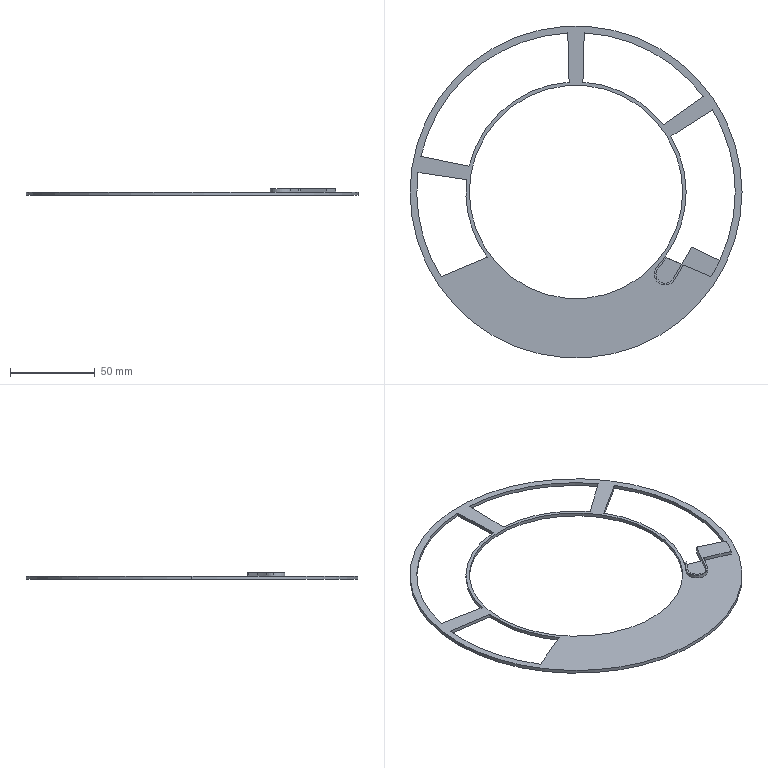Part | SolidWorks | features ICE 4, Extrusion 1, Fillet 1 | 1 solid | 39 faces | box 196 x 196 x 4 mm | volume 17953 mm3 | cylinder 23 | plane 16 | commonest cylinder face diameters 130 x6 188 x6 2 x2 10.964 x2 12.964 x2 126 x2
STEP:
#1=CARTESIAN_POINT('',(46.182,-48.334,4.));
#2=VERTEX_POINT('',#1);
#3=CARTESIAN_POINT('',(58.26,-51.606,4.));
#4=VERTEX_POINT('',#3);
#5=CARTESIAN_POINT('',(52.665,-48.334,4.));
#6=DIRECTION('',(0.,0.,1.));
#7=DIRECTION('',(1.,0.,0.));
#8=AXIS2_PLACEMENT_3D('',#5,#6,#7);
#9=CIRCLE('',#8,6.482);
#10=EDGE_CURVE('',#2,#4,#9,.T.);
#11=ORIENTED_EDGE('',*,*,#10,.F.);
#12=CARTESIAN_POINT('',(46.182,-48.334,2.));
#13=VERTEX_POINT('',#12);
#14=CARTESIAN_POINT('',(46.182,-48.334,4.));
#15=DIRECTION('',(0.,0.,-1.));
#16=VECTOR('',#15,1000.);
#17=LINE('',#14,#16);
#18=EDGE_CURVE('',#2,#13,#17,.T.);
#19=ORIENTED_EDGE('',*,*,#18,.T.);
#20=CARTESIAN_POINT('',(58.26,-51.606,2.));
#21=VERTEX_POINT('',#20);
#22=CARTESIAN_POINT('',(52.665,-48.334,2.));
#23=DIRECTION('',(0.,0.,-1.));
#24=DIRECTION('',(1.,0.,0.));
#25=AXIS2_PLACEMENT_3D('',#22,#23,#24);
#26=CIRCLE('',#25,6.482);
#27=EDGE_CURVE('',#21,#13,#26,.T.);
#28=ORIENTED_EDGE('',*,*,#27,.F.);
#29=CARTESIAN_POINT('',(58.26,-51.606,4.));
#30=DIRECTION('',(0.,0.,-1.));
#31=VECTOR('',#30,1000.);
#32=LINE('',#29,#31);
#33=EDGE_CURVE('',#4,#21,#32,.T.);
#34=ORIENTED_EDGE('',*,*,#33,.F.);
#35=EDGE_LOOP('',(#11,#19,#28,#34));
#36=FACE_OUTER_BOUND('',#35,.T.);
#37=CARTESIAN_POINT('',(52.665,-48.334,4.));
#38=DIRECTION('',(0.,0.,-1.));
#39=DIRECTION('',(-1.,0.,0.));
#40=AXIS2_PLACEMENT_3D('',#37,#38,#39);
#41=CYLINDRICAL_SURFACE('',#40,6.482);
#42=ADVANCED_FACE('',(#36),#41,.T.);
#43=CARTESIAN_POINT('',(48.626,-44.627,4.));
#44=VERTEX_POINT('',#43);
#45=CARTESIAN_POINT('',(47.182,-48.334,4.));
#46=VERTEX_POINT('',#45);
#47=CARTESIAN_POINT('',(52.665,-48.334,4.));
#48=DIRECTION('',(0.,0.,1.));
#49=DIRECTION('',(1.,0.,0.));
#50=AXIS2_PLACEMENT_3D('',#47,#48,#49);
#51=CIRCLE('',#50,5.482);
#52=EDGE_CURVE('',#44,#46,#51,.T.);
#53=ORIENTED_EDGE('',*,*,#52,.T.);
#54=CARTESIAN_POINT('',(47.182,-48.334,2.));
#55=VERTEX_POINT('',#54);
#56=CARTESIAN_POINT('',(47.182,-48.334,4.));
#57=DIRECTION('',(0.,0.,-1.));
#58=VECTOR('',#57,1000.);
#59=LINE('',#56,#58);
#60=EDGE_CURVE('',#46,#55,#59,.T.);
#61=ORIENTED_EDGE('',*,*,#60,.T.);
#62=CARTESIAN_POINT('',(48.626,-44.627,2.));
#63=VERTEX_POINT('',#62);
#64=CARTESIAN_POINT('',(52.665,-48.334,2.));
#65=DIRECTION('',(0.,0.,-1.));
#66=DIRECTION('',(1.,0.,0.));
#67=AXIS2_PLACEMENT_3D('',#64,#65,#66);
#68=CIRCLE('',#67,5.482);
#69=EDGE_CURVE('',#55,#63,#68,.T.);
#70=ORIENTED_EDGE('',*,*,#69,.T.);
#71=CARTESIAN_POINT('',(48.626,-44.627,4.));
#72=DIRECTION('',(0.,0.,-1.));
#73=VECTOR('',#72,1000.);
#74=LINE('',#71,#73);
#75=EDGE_CURVE('',#44,#63,#74,.T.);
#76=ORIENTED_EDGE('',*,*,#75,.F.);
#77=EDGE_LOOP('',(#53,#61,#70,#76));
#78=FACE_OUTER_BOUND('',#77,.T.);
#79=CARTESIAN_POINT('',(52.665,-48.334,4.));
#80=DIRECTION('',(0.,0.,-1.));
#81=DIRECTION('',(-1.,0.,0.));
#82=AXIS2_PLACEMENT_3D('',#79,#80,#81);
#83=CYLINDRICAL_SURFACE('',#82,5.482);
#84=ADVANCED_FACE('',(#78),#83,.F.);
#85=CARTESIAN_POINT('',(-63.,0.,2.));
#86=VERTEX_POINT('',#85);
#87=CARTESIAN_POINT('',(63.,0.,2.));
#88=VERTEX_POINT('',#87);
#89=CARTESIAN_POINT('',(0.,0.,2.));
#90=DIRECTION('',(0.,0.,1.));
#91=DIRECTION('',(1.,0.,0.));
#92=AXIS2_PLACEMENT_3D('',#89,#90,#91);
#93=CIRCLE('',#92,63.);
#94=EDGE_CURVE('',#86,#88,#93,.T.);
#95=ORIENTED_EDGE('',*,*,#94,.T.);
#96=CARTESIAN_POINT('',(63.,0.,0.));
#97=VERTEX_POINT('',#96);
#98=CARTESIAN_POINT('',(63.,0.,2.));
#99=DIRECTION('',(0.,0.,-1.));
#100=VECTOR('',#99,1000.);
#101=LINE('',#98,#100);
#102=EDGE_CURVE('',#88,#97,#101,.T.);
#103=ORIENTED_EDGE('',*,*,#102,.T.);
#104=CARTESIAN_POINT('',(-63.,0.,0.));
#105=VERTEX_POINT('',#104);
#106=CARTESIAN_POINT('',(0.,0.,0.));
#107=DIRECTION('',(0.,0.,1.));
#108=DIRECTION('',(1.,0.,0.));
#109=AXIS2_PLACEMENT_3D('',#106,#107,#108);
#110=CIRCLE('',#109,63.);
#111=EDGE_CURVE('',#105,#97,#110,.T.);
#112=ORIENTED_EDGE('',*,*,#111,.F.);
#113=CARTESIAN_POINT('',(-63.,0.,2.));
#114=DIRECTION('',(0.,0.,-1.));
#115=VECTOR('',#114,1000.);
#116=LINE('',#113,#115);
#117=EDGE_CURVE('',#86,#105,#116,.T.);
#118=ORIENTED_EDGE('',*,*,#117,.F.);
#119=EDGE_LOOP('',(#95,#103,#112,#118));
#120=FACE_OUTER_BOUND('',#119,.T.);
#121=CARTESIAN_POINT('',(0.,0.,2.));
#122=DIRECTION('',(0.,0.,-1.));
#123=DIRECTION('',(-1.,0.,0.));
#124=AXIS2_PLACEMENT_3D('',#121,#122,#123);
#125=CYLINDRICAL_SURFACE('',#124,63.);
#126=ADVANCED_FACE('',(#120),#125,.F.);
#127=CARTESIAN_POINT('',(98.,0.,2.));
#128=VERTEX_POINT('',#127);
#129=CARTESIAN_POINT('',(-98.,0.,2.));
#130=VERTEX_POINT('',#129);
#131=CARTESIAN_POINT('',(0.,0.,2.));
#132=DIRECTION('',(0.,0.,1.));
#133=DIRECTION('',(1.,0.,0.));
#134=AXIS2_PLACEMENT_3D('',#131,#132,#133);
#135=CIRCLE('',#134,98.);
#136=EDGE_CURVE('',#128,#130,#135,.T.);
#137=ORIENTED_EDGE('',*,*,#136,.F.);
#138=CARTESIAN_POINT('',(98.,0.,0.));
#139=VERTEX_POINT('',#138);
#140=CARTESIAN_POINT('',(98.,0.,2.));
#141=DIRECTION('',(0.,0.,-1.));
#142=VECTOR('',#141,1000.);
#143=LINE('',#140,#142);
#144=EDGE_CURVE('',#128,#139,#143,.T.);
#145=ORIENTED_EDGE('',*,*,#144,.T.);
#146=CARTESIAN_POINT('',(-98.,0.,0.));
#147=VERTEX_POINT('',#146);
#148=CARTESIAN_POINT('',(0.,0.,0.));
#149=DIRECTION('',(0.,0.,1.));
#150=DIRECTION('',(1.,0.,0.));
#151=AXIS2_PLACEMENT_3D('',#148,#149,#150);
#152=CIRCLE('',#151,98.);
#153=EDGE_CURVE('',#139,#147,#152,.T.);
#154=ORIENTED_EDGE('',*,*,#153,.T.);
#155=CARTESIAN_POINT('',(-98.,0.,2.));
#156=DIRECTION('',(0.,0.,-1.));
#157=VECTOR('',#156,1000.);
#158=LINE('',#155,#157);
#159=EDGE_CURVE('',#130,#147,#158,.T.);
#160=ORIENTED_EDGE('',*,*,#159,.F.);
#161=EDGE_LOOP('',(#137,#145,#154,#160));
#162=FACE_OUTER_BOUND('',#161,.T.);
#163=CARTESIAN_POINT('',(0.,0.,2.));
#164=DIRECTION('',(0.,0.,-1.));
#165=DIRECTION('',(-1.,0.,0.));
#166=AXIS2_PLACEMENT_3D('',#163,#164,#165);
#167=CYLINDRICAL_SURFACE('',#166,98.);
#168=ADVANCED_FACE('',(#162),#167,.T.);
#169=CARTESIAN_POINT('',(52.424,-38.428,0.));
#170=VERTEX_POINT('',#169);
#171=CARTESIAN_POINT('',(65.,0.,0.));
#172=VERTEX_POINT('',#171);
#173=CARTESIAN_POINT('',(0.,0.,0.));
#174=DIRECTION('',(0.,0.,1.));
#175=DIRECTION('',(1.,0.,0.));
#176=AXIS2_PLACEMENT_3D('',#173,#174,#175);
#177=CIRCLE('',#176,65.);
#178=EDGE_CURVE('',#170,#172,#177,.T.);
#179=ORIENTED_EDGE('',*,*,#178,.T.);
#180=CARTESIAN_POINT('',(65.,0.,2.));
#181=VERTEX_POINT('',#180);
#182=CARTESIAN_POINT('',(65.,0.,-3.));
#183=DIRECTION('',(0.,0.,1.));
#184=VECTOR('',#183,1000.);
#185=LINE('',#182,#184);
#186=EDGE_CURVE('',#172,#181,#185,.T.);
#187=ORIENTED_EDGE('',*,*,#186,.T.);
#188=CARTESIAN_POINT('',(52.424,-38.428,2.));
#189=VERTEX_POINT('',#188);
#190=CARTESIAN_POINT('',(0.,0.,2.));
#191=DIRECTION('',(0.,0.,1.));
#192=DIRECTION('',(1.,0.,0.));
#193=AXIS2_PLACEMENT_3D('',#190,#191,#192);
#194=CIRCLE('',#193,65.);
#195=EDGE_CURVE('',#189,#181,#194,.T.);
#196=ORIENTED_EDGE('',*,*,#195,.F.);
#197=CARTESIAN_POINT('',(52.424,-38.428,0.));
#198=DIRECTION('',(0.,0.,1.));
#199=VECTOR('',#198,1000.);
#200=LINE('',#197,#199);
#201=EDGE_CURVE('',#170,#189,#200,.T.);
#202=ORIENTED_EDGE('',*,*,#201,.F.);
#203=EDGE_LOOP('',(#179,#187,#196,#202));
#204=FACE_OUTER_BOUND('',#203,.T.);
#205=CARTESIAN_POINT('',(0.,0.,-3.));
#206=DIRECTION('',(0.,0.,1.));
#207=DIRECTION('',(1.,0.,0.));
#208=AXIS2_PLACEMENT_3D('',#205,#206,#207);
#209=CYLINDRICAL_SURFACE('',#208,65.);
#210=ADVANCED_FACE('',(#204),#209,.T.);
#211=CARTESIAN_POINT('',(94.,0.,0.));
#212=VERTEX_POINT('',#211);
#213=CARTESIAN_POINT('',(80.531,48.485,0.));
#214=VERTEX_POINT('',#213);
#215=CARTESIAN_POINT('',(0.,0.,0.));
#216=DIRECTION('',(0.,0.,1.));
#217=DIRECTION('',(1.,0.,0.));
#218=AXIS2_PLACEMENT_3D('',#215,#216,#217);
#219=CIRCLE('',#218,94.);
#220=EDGE_CURVE('',#212,#214,#219,.T.);
#221=ORIENTED_EDGE('',*,*,#220,.F.);
#222=CARTESIAN_POINT('',(94.,0.,2.));
#223=VERTEX_POINT('',#222);
#224=CARTESIAN_POINT('',(94.,0.,-3.));
#225=DIRECTION('',(0.,0.,1.));
#226=VECTOR('',#225,1000.);
#227=LINE('',#224,#226);
#228=EDGE_CURVE('',#212,#223,#227,.T.);
#229=ORIENTED_EDGE('',*,*,#228,.T.);
#230=CARTESIAN_POINT('',(80.531,48.485,2.));
#231=VERTEX_POINT('',#230);
#232=CARTESIAN_POINT('',(0.,0.,2.));
#233=DIRECTION('',(0.,0.,1.));
#234=DIRECTION('',(1.,0.,0.));
#235=AXIS2_PLACEMENT_3D('',#232,#233,#234);
#236=CIRCLE('',#235,94.);
#237=EDGE_CURVE('',#223,#231,#236,.T.);
#238=ORIENTED_EDGE('',*,*,#237,.T.);
#239=CARTESIAN_POINT('',(80.531,48.485,0.));
#240=DIRECTION('',(0.,0.,1.));
#241=VECTOR('',#240,1000.);
#242=LINE('',#239,#241);
#243=EDGE_CURVE('',#214,#231,#242,.T.);
#244=ORIENTED_EDGE('',*,*,#243,.F.);
#245=EDGE_LOOP('',(#221,#229,#238,#244));
#246=FACE_OUTER_BOUND('',#245,.T.);
#247=CARTESIAN_POINT('',(0.,0.,-3.));
#248=DIRECTION('',(0.,0.,1.));
#249=DIRECTION('',(1.,0.,0.));
#250=AXIS2_PLACEMENT_3D('',#247,#248,#249);
#251=CYLINDRICAL_SURFACE('',#250,94.);
#252=ADVANCED_FACE('',(#246),#251,.F.);
#253=CARTESIAN_POINT('',(62.357,-42.62,2.));
#254=VERTEX_POINT('',#253);
#255=CARTESIAN_POINT('',(57.397,-51.101,2.));
#256=VERTEX_POINT('',#255);
#257=CARTESIAN_POINT('',(65.037,-38.039,2.));
#258=DIRECTION('',(-0.5049,-0.8632,0.));
#259=VECTOR('',#258,1000.);
#260=LINE('',#257,#259);
#261=EDGE_CURVE('',#254,#256,#260,.T.);
#262=ORIENTED_EDGE('',*,*,#261,.F.);
#263=CARTESIAN_POINT('',(53.371,-38.828,2.));
#264=VERTEX_POINT('',#263);
#265=CARTESIAN_POINT('',(52.424,-38.428,2.));
#266=DIRECTION('',(-0.9213,0.3888,0.));
#267=VECTOR('',#266,1000.);
#268=LINE('',#265,#267);
#269=EDGE_CURVE('',#254,#264,#268,.T.);
#270=ORIENTED_EDGE('',*,*,#269,.T.);
#271=CARTESIAN_POINT('',(0.,0.,2.));
#272=DIRECTION('',(0.,0.,-1.));
#273=DIRECTION('',(1.,0.,0.));
#274=AXIS2_PLACEMENT_3D('',#271,#272,#273);
#275=CIRCLE('',#274,66.);
#276=EDGE_CURVE('',#264,#63,#275,.T.);
#277=ORIENTED_EDGE('',*,*,#276,.T.);
#278=ORIENTED_EDGE('',*,*,#69,.F.);
#279=CARTESIAN_POINT('',(52.665,-48.334,2.));
#280=DIRECTION('',(0.,0.,-1.));
#281=DIRECTION('',(1.,0.,0.));
#282=AXIS2_PLACEMENT_3D('',#279,#280,#281);
#283=CIRCLE('',#282,5.482);
#284=EDGE_CURVE('',#256,#55,#283,.T.);
#285=ORIENTED_EDGE('',*,*,#284,.F.);
#286=EDGE_LOOP('',(#262,#270,#277,#278,#285));
#287=FACE_OUTER_BOUND('',#286,.T.);
#288=CARTESIAN_POINT('',(0.,0.,2.));
#289=DIRECTION('',(0.,0.,1.));
#290=DIRECTION('',(1.,0.,0.));
#291=AXIS2_PLACEMENT_3D('',#288,#289,#290);
#292=PLANE('',#291);
#293=ADVANCED_FACE('',(#287),#292,.T.);
#294=ORIENTED_EDGE('',*,*,#228,.F.);
#295=CARTESIAN_POINT('',(84.854,-40.445,0.));
#296=VERTEX_POINT('',#295);
#297=CARTESIAN_POINT('',(0.,0.,0.));
#298=DIRECTION('',(0.,0.,1.));
#299=DIRECTION('',(1.,0.,0.));
#300=AXIS2_PLACEMENT_3D('',#297,#298,#299);
#301=CIRCLE('',#300,94.);
#302=EDGE_CURVE('',#296,#212,#301,.T.);
#303=ORIENTED_EDGE('',*,*,#302,.F.);
#304=CARTESIAN_POINT('',(84.854,-40.445,2.));
#305=VERTEX_POINT('',#304);
#306=CARTESIAN_POINT('',(84.854,-40.445,4.));
#307=DIRECTION('',(0.,0.,-1.));
#308=VECTOR('',#307,1000.);
#309=LINE('',#306,#308);
#310=EDGE_CURVE('',#305,#296,#309,.T.);
#311=ORIENTED_EDGE('',*,*,#310,.F.);
#312=CARTESIAN_POINT('',(0.,0.,2.));
#313=DIRECTION('',(0.,0.,1.));
#314=DIRECTION('',(1.,0.,0.));
#315=AXIS2_PLACEMENT_3D('',#312,#313,#314);
#316=CIRCLE('',#315,94.);
#317=EDGE_CURVE('',#305,#223,#316,.T.);
#318=ORIENTED_EDGE('',*,*,#317,.T.);
#319=EDGE_LOOP('',(#294,#303,#311,#318));
#320=FACE_OUTER_BOUND('',#319,.T.);
#321=CARTESIAN_POINT('',(0.,0.,-3.));
#322=DIRECTION('',(0.,0.,1.));
#323=DIRECTION('',(1.,0.,0.));
#324=AXIS2_PLACEMENT_3D('',#321,#322,#323);
#325=CYLINDRICAL_SURFACE('',#324,94.);
#326=ADVANCED_FACE('',(#320),#325,.F.);
#327=ORIENTED_EDGE('',*,*,#186,.F.);
#328=CARTESIAN_POINT('',(56.061,32.896,0.));
#329=VERTEX_POINT('',#328);
#330=CARTESIAN_POINT('',(0.,0.,0.));
#331=DIRECTION('',(0.,0.,1.));
#332=DIRECTION('',(1.,0.,0.));
#333=AXIS2_PLACEMENT_3D('',#330,#331,#332);
#334=CIRCLE('',#333,65.);
#335=EDGE_CURVE('',#172,#329,#334,.T.);
#336=ORIENTED_EDGE('',*,*,#335,.T.);
#337=CARTESIAN_POINT('',(56.061,32.896,2.));
#338=VERTEX_POINT('',#337);
#339=CARTESIAN_POINT('',(56.061,32.896,0.));
#340=DIRECTION('',(0.,0.,1.));
#341=VECTOR('',#340,1000.);
#342=LINE('',#339,#341);
#343=EDGE_CURVE('',#329,#338,#342,.T.);
#344=ORIENTED_EDGE('',*,*,#343,.T.);
#345=CARTESIAN_POINT('',(0.,0.,2.));
#346=DIRECTION('',(0.,0.,1.));
#347=DIRECTION('',(1.,0.,0.));
#348=AXIS2_PLACEMENT_3D('',#345,#346,#347);
#349=CIRCLE('',#348,65.);
#350=EDGE_CURVE('',#181,#338,#349,.T.);
#351=ORIENTED_EDGE('',*,*,#350,.F.);
#352=EDGE_LOOP('',(#327,#336,#344,#351));
#353=FACE_OUTER_BOUND('',#352,.T.);
#354=CARTESIAN_POINT('',(0.,0.,-3.));
#355=DIRECTION('',(0.,0.,1.));
#356=DIRECTION('',(1.,0.,0.));
#357=AXIS2_PLACEMENT_3D('',#354,#355,#356);
#358=CYLINDRICAL_SURFACE('',#357,65.);
#359=ADVANCED_FACE('',(#353),#358,.T.);
#360=CARTESIAN_POINT('',(-4.836,93.876,2.));
#361=VERTEX_POINT('',#360);
#362=CARTESIAN_POINT('',(-91.61,21.064,2.));
#363=VERTEX_POINT('',#362);
#364=CARTESIAN_POINT('',(0.,0.,2.));
#365=DIRECTION('',(0.,0.,1.));
#366=DIRECTION('',(1.,0.,0.));
#367=AXIS2_PLACEMENT_3D('',#364,#365,#366);
#368=CIRCLE('',#367,94.);
#369=EDGE_CURVE('',#361,#363,#368,.T.);
#370=ORIENTED_EDGE('',*,*,#369,.T.);
#371=CARTESIAN_POINT('',(-91.61,21.064,0.));
#372=VERTEX_POINT('',#371);
#373=CARTESIAN_POINT('',(-91.61,21.064,0.));
#374=DIRECTION('',(0.,0.,1.));
#375=VECTOR('',#374,1000.);
#376=LINE('',#373,#375);
#377=EDGE_CURVE('',#372,#363,#376,.T.);
#378=ORIENTED_EDGE('',*,*,#377,.F.);
#379=CARTESIAN_POINT('',(-4.836,93.876,0.));
#380=VERTEX_POINT('',#379);
#381=CARTESIAN_POINT('',(0.,0.,0.));
#382=DIRECTION('',(0.,0.,1.));
#383=DIRECTION('',(1.,0.,0.));
#384=AXIS2_PLACEMENT_3D('',#381,#382,#383);
#385=CIRCLE('',#384,94.);
#386=EDGE_CURVE('',#380,#372,#385,.T.);
#387=ORIENTED_EDGE('',*,*,#386,.F.);
#388=CARTESIAN_POINT('',(-4.836,93.876,0.));
#389=DIRECTION('',(0.,0.,1.));
#390=VECTOR('',#389,1000.);
#391=LINE('',#388,#390);
#392=EDGE_CURVE('',#380,#361,#391,.T.);
#393=ORIENTED_EDGE('',*,*,#392,.T.);
#394=EDGE_LOOP('',(#370,#378,#387,#393));
#395=FACE_OUTER_BOUND('',#394,.T.);
#396=CARTESIAN_POINT('',(0.,0.,-3.));
#397=DIRECTION('',(0.,0.,1.));
#398=DIRECTION('',(1.,0.,0.));
#399=AXIS2_PLACEMENT_3D('',#396,#397,#398);
#400=CYLINDRICAL_SURFACE('',#399,94.);
#401=ADVANCED_FACE('',(#395),#400,.F.);
#402=CARTESIAN_POINT('',(-63.179,15.28,0.));
#403=VERTEX_POINT('',#402);
#404=CARTESIAN_POINT('',(-63.179,15.28,2.));
#405=VERTEX_POINT('',#404);
#406=CARTESIAN_POINT('',(-63.179,15.28,0.));
#407=DIRECTION('',(0.,0.,1.));
#408=VECTOR('',#407,1000.);
#409=LINE('',#406,#408);
#410=EDGE_CURVE('',#403,#405,#409,.T.);
#411=ORIENTED_EDGE('',*,*,#410,.T.);
#412=CARTESIAN_POINT('',(-4.077,64.872,2.));
#413=VERTEX_POINT('',#412);
#414=CARTESIAN_POINT('',(0.,0.,2.));
#415=DIRECTION('',(0.,0.,1.));
#416=DIRECTION('',(1.,0.,0.));
#417=AXIS2_PLACEMENT_3D('',#414,#415,#416);
#418=CIRCLE('',#417,65.);
#419=EDGE_CURVE('',#413,#405,#418,.T.);
#420=ORIENTED_EDGE('',*,*,#419,.F.);
#421=CARTESIAN_POINT('',(-4.077,64.872,0.));
#422=VERTEX_POINT('',#421);
#423=CARTESIAN_POINT('',(-4.077,64.872,0.));
#424=DIRECTION('',(0.,0.,1.));
#425=VECTOR('',#424,1000.);
#426=LINE('',#423,#425);
#427=EDGE_CURVE('',#422,#413,#426,.T.);
#428=ORIENTED_EDGE('',*,*,#427,.F.);
#429=CARTESIAN_POINT('',(0.,0.,0.));
#430=DIRECTION('',(0.,0.,1.));
#431=DIRECTION('',(1.,0.,0.));
#432=AXIS2_PLACEMENT_3D('',#429,#430,#431);
#433=CIRCLE('',#432,65.);
#434=EDGE_CURVE('',#422,#403,#433,.T.);
#435=ORIENTED_EDGE('',*,*,#434,.T.);
#436=EDGE_LOOP('',(#411,#420,#428,#435));
#437=FACE_OUTER_BOUND('',#436,.T.);
#438=CARTESIAN_POINT('',(0.,0.,-3.));
#439=DIRECTION('',(0.,0.,1.));
#440=DIRECTION('',(1.,0.,0.));
#441=AXIS2_PLACEMENT_3D('',#438,#439,#440);
#442=CYLINDRICAL_SURFACE('',#441,65.);
#443=ADVANCED_FACE('',(#437),#442,.T.);
#444=CARTESIAN_POINT('',(-93.289,11.539,2.));
#445=VERTEX_POINT('',#444);
#446=CARTESIAN_POINT('',(-79.65,-49.919,2.));
#447=VERTEX_POINT('',#446);
#448=CARTESIAN_POINT('',(0.,0.,2.));
#449=DIRECTION('',(0.,0.,1.));
#450=DIRECTION('',(1.,0.,0.));
#451=AXIS2_PLACEMENT_3D('',#448,#449,#450);
#452=CIRCLE('',#451,94.);
#453=EDGE_CURVE('',#445,#447,#452,.T.);
#454=ORIENTED_EDGE('',*,*,#453,.T.);
#455=CARTESIAN_POINT('',(-79.65,-49.919,0.));
#456=VERTEX_POINT('',#455);
#457=CARTESIAN_POINT('',(-79.65,-49.919,0.));
#458=DIRECTION('',(0.,0.,1.));
#459=VECTOR('',#458,1000.);
#460=LINE('',#457,#459);
#461=EDGE_CURVE('',#456,#447,#460,.T.);
#462=ORIENTED_EDGE('',*,*,#461,.F.);
#463=CARTESIAN_POINT('',(-93.289,11.539,0.));
#464=VERTEX_POINT('',#463);
#465=CARTESIAN_POINT('',(0.,0.,0.));
#466=DIRECTION('',(0.,0.,1.));
#467=DIRECTION('',(1.,0.,0.));
#468=AXIS2_PLACEMENT_3D('',#465,#466,#467);
#469=CIRCLE('',#468,94.);
#470=EDGE_CURVE('',#464,#456,#469,.T.);
#471=ORIENTED_EDGE('',*,*,#470,.F.);
#472=CARTESIAN_POINT('',(-93.289,11.539,0.));
#473=DIRECTION('',(0.,0.,1.));
#474=VECTOR('',#473,1000.);
#475=LINE('',#472,#474);
#476=EDGE_CURVE('',#464,#445,#475,.T.);
#477=ORIENTED_EDGE('',*,*,#476,.T.);
#478=EDGE_LOOP('',(#454,#462,#471,#477));
#479=FACE_OUTER_BOUND('',#478,.T.);
#480=CARTESIAN_POINT('',(0.,0.,-3.));
#481=DIRECTION('',(0.,0.,1.));
#482=DIRECTION('',(1.,0.,0.));
#483=AXIS2_PLACEMENT_3D('',#480,#481,#482);
#484=CYLINDRICAL_SURFACE('',#483,94.);
#485=ADVANCED_FACE('',(#479),#484,.F.);
#486=CARTESIAN_POINT('',(-52.424,-38.428,0.));
#487=VERTEX_POINT('',#486);
#488=CARTESIAN_POINT('',(-52.424,-38.428,2.));
#489=VERTEX_POINT('',#488);
#490=CARTESIAN_POINT('',(-52.424,-38.428,0.));
#491=DIRECTION('',(0.,0.,1.));
#492=VECTOR('',#491,1000.);
#493=LINE('',#490,#492);
#494=EDGE_CURVE('',#487,#489,#493,.T.);
#495=ORIENTED_EDGE('',*,*,#494,.T.);
#496=CARTESIAN_POINT('',(-64.594,7.25,2.));
#497=VERTEX_POINT('',#496);
#498=CARTESIAN_POINT('',(0.,0.,2.));
#499=DIRECTION('',(0.,0.,1.));
#500=DIRECTION('',(1.,0.,0.));
#501=AXIS2_PLACEMENT_3D('',#498,#499,#500);
#502=CIRCLE('',#501,65.);
#503=EDGE_CURVE('',#497,#489,#502,.T.);
#504=ORIENTED_EDGE('',*,*,#503,.F.);
#505=CARTESIAN_POINT('',(-64.594,7.25,0.));
#506=VERTEX_POINT('',#505);
#507=CARTESIAN_POINT('',(-64.594,7.25,0.));
#508=DIRECTION('',(0.,0.,1.));
#509=VECTOR('',#508,1000.);
#510=LINE('',#507,#509);
#511=EDGE_CURVE('',#506,#497,#510,.T.);
#512=ORIENTED_EDGE('',*,*,#511,.F.);
#513=CARTESIAN_POINT('',(0.,0.,0.));
#514=DIRECTION('',(0.,0.,1.));
#515=DIRECTION('',(1.,0.,0.));
#516=AXIS2_PLACEMENT_3D('',#513,#514,#515);
#517=CIRCLE('',#516,65.);
#518=EDGE_CURVE('',#506,#487,#517,.T.);
#519=ORIENTED_EDGE('',*,*,#518,.T.);
#520=EDGE_LOOP('',(#495,#504,#512,#519));
#521=FACE_OUTER_BOUND('',#520,.T.);
#522=CARTESIAN_POINT('',(0.,0.,-3.));
#523=DIRECTION('',(0.,0.,1.));
#524=DIRECTION('',(1.,0.,0.));
#525=AXIS2_PLACEMENT_3D('',#522,#523,#524);
#526=CYLINDRICAL_SURFACE('',#525,65.);
#527=ADVANCED_FACE('',(#521),#526,.T.);
#528=CARTESIAN_POINT('',(79.65,-49.919,2.));
#529=VERTEX_POINT('',#528);
#530=CARTESIAN_POINT('',(64.095,-43.354,2.));
#531=VERTEX_POINT('',#530);
#532=CARTESIAN_POINT('',(52.424,-38.428,2.));
#533=DIRECTION('',(-0.9213,0.3888,0.));
#534=VECTOR('',#533,1000.);
#535=LINE('',#532,#534);
#536=EDGE_CURVE('',#529,#531,#535,.T.);
#537=ORIENTED_EDGE('',*,*,#536,.T.);
#538=CARTESIAN_POINT('',(62.843,-43.77,2.));
#539=VERTEX_POINT('',#538);
#540=CARTESIAN_POINT('',(63.706,-44.275,2.));
#541=DIRECTION('',(0.,0.,1.));
#542=DIRECTION('',(1.,0.,0.));
#543=AXIS2_PLACEMENT_3D('',#540,#541,#542);
#544=CIRCLE('',#543,1.);
#545=EDGE_CURVE('',#531,#539,#544,.T.);
#546=ORIENTED_EDGE('',*,*,#545,.T.);
#547=CARTESIAN_POINT('',(65.9,-38.544,2.));
#548=DIRECTION('',(-0.5049,-0.8632,0.));
#549=VECTOR('',#548,1000.);
#550=LINE('',#547,#549);
#551=EDGE_CURVE('',#539,#21,#550,.T.);
#552=ORIENTED_EDGE('',*,*,#551,.T.);
#553=ORIENTED_EDGE('',*,*,#27,.T.);
#554=CARTESIAN_POINT('',(47.889,-43.951,2.));
#555=VERTEX_POINT('',#554);
#556=CARTESIAN_POINT('',(52.665,-48.334,2.));
#557=DIRECTION('',(0.,0.,-1.));
#558=DIRECTION('',(1.,0.,0.));
#559=AXIS2_PLACEMENT_3D('',#556,#557,#558);
#560=CIRCLE('',#559,6.482);
#561=EDGE_CURVE('',#13,#555,#560,.T.);
#562=ORIENTED_EDGE('',*,*,#561,.T.);
#563=CARTESIAN_POINT('',(0.,0.,2.));
#564=DIRECTION('',(0.,0.,-1.));
#565=DIRECTION('',(1.,0.,0.));
#566=AXIS2_PLACEMENT_3D('',#563,#564,#565);
#567=CIRCLE('',#566,65.);
#568=EDGE_CURVE('',#189,#555,#567,.T.);
#569=ORIENTED_EDGE('',*,*,#568,.F.);
#570=ORIENTED_EDGE('',*,*,#195,.T.);
#571=ORIENTED_EDGE('',*,*,#350,.T.);
#572=CARTESIAN_POINT('',(80.531,48.485,2.));
#573=DIRECTION('',(0.8434,0.5373,0.));
#574=VECTOR('',#573,1000.);
#575=LINE('',#572,#574);
#576=EDGE_CURVE('',#338,#231,#575,.T.);
#577=ORIENTED_EDGE('',*,*,#576,.T.);
#578=ORIENTED_EDGE('',*,*,#237,.F.);
#579=ORIENTED_EDGE('',*,*,#317,.F.);
#580=CARTESIAN_POINT('',(0.,0.,2.));
#581=DIRECTION('',(0.,0.,1.));
#582=DIRECTION('',(1.,0.,0.));
#583=AXIS2_PLACEMENT_3D('',#580,#581,#582);
#584=CIRCLE('',#583,94.);
#585=EDGE_CURVE('',#529,#305,#584,.T.);
#586=ORIENTED_EDGE('',*,*,#585,.F.);
#587=EDGE_LOOP('',(#537,#546,#552,#553,#562,#569,#570,#571,#577,#578,#579,#586));
#588=FACE_BOUND('',#587,.T.);
#589=ORIENTED_EDGE('',*,*,#503,.T.);
#590=CARTESIAN_POINT('',(-52.424,-38.428,2.));
#591=DIRECTION('',(-0.9213,-0.3888,0.));
#592=VECTOR('',#591,1000.);
#593=LINE('',#590,#592);
#594=EDGE_CURVE('',#489,#447,#593,.T.);
#595=ORIENTED_EDGE('',*,*,#594,.T.);
#596=ORIENTED_EDGE('',*,*,#453,.F.);
#597=CARTESIAN_POINT('',(-93.289,11.539,2.));
#598=DIRECTION('',(0.989,-0.1478,0.));
#599=VECTOR('',#598,1000.);
#600=LINE('',#597,#599);
#601=EDGE_CURVE('',#445,#497,#600,.T.);
#602=ORIENTED_EDGE('',*,*,#601,.T.);
#603=EDGE_LOOP('',(#589,#595,#596,#602));
#604=FACE_BOUND('',#603,.T.);
#605=CARTESIAN_POINT('',(75.122,56.504,2.));
#606=VERTEX_POINT('',#605);
#607=CARTESIAN_POINT('',(4.836,93.876,2.));
#608=VERTEX_POINT('',#607);
#609=CARTESIAN_POINT('',(0.,0.,2.));
#610=DIRECTION('',(0.,0.,1.));
#611=DIRECTION('',(1.,0.,0.));
#612=AXIS2_PLACEMENT_3D('',#609,#610,#611);
#613=CIRCLE('',#612,94.);
#614=EDGE_CURVE('',#606,#608,#613,.T.);
#615=ORIENTED_EDGE('',*,*,#614,.F.);
#616=CARTESIAN_POINT('',(51.502,39.656,2.));
#617=VERTEX_POINT('',#616);
#618=CARTESIAN_POINT('',(75.122,56.504,2.));
#619=DIRECTION('',(-0.8141,-0.5807,0.));
#620=VECTOR('',#619,1000.);
#621=LINE('',#618,#620);
#622=EDGE_CURVE('',#606,#617,#621,.T.);
#623=ORIENTED_EDGE('',*,*,#622,.T.);
#624=CARTESIAN_POINT('',(4.077,64.872,2.));
#625=VERTEX_POINT('',#624);
#626=CARTESIAN_POINT('',(0.,0.,2.));
#627=DIRECTION('',(0.,0.,1.));
#628=DIRECTION('',(1.,0.,0.));
#629=AXIS2_PLACEMENT_3D('',#626,#627,#628);
#630=CIRCLE('',#629,65.);
#631=EDGE_CURVE('',#617,#625,#630,.T.);
#632=ORIENTED_EDGE('',*,*,#631,.T.);
#633=CARTESIAN_POINT('',(4.836,93.876,2.));
#634=DIRECTION('',(0.02618,0.9997,0.));
#635=VECTOR('',#634,1000.);
#636=LINE('',#633,#635);
#637=EDGE_CURVE('',#625,#608,#636,.T.);
#638=ORIENTED_EDGE('',*,*,#637,.T.);
#639=EDGE_LOOP('',(#615,#623,#632,#638));
#640=FACE_BOUND('',#639,.T.);
#641=ORIENTED_EDGE('',*,*,#369,.F.);
#642=CARTESIAN_POINT('',(-4.836,93.876,2.));
#643=DIRECTION('',(0.02618,-0.9997,0.));
#644=VECTOR('',#643,1000.);
#645=LINE('',#642,#644);
#646=EDGE_CURVE('',#361,#413,#645,.T.);
#647=ORIENTED_EDGE('',*,*,#646,.T.);
#648=ORIENTED_EDGE('',*,*,#419,.T.);
#649=CARTESIAN_POINT('',(-91.61,21.064,2.));
#650=DIRECTION('',(-0.9799,0.1994,0.));
#651=VECTOR('',#650,1000.);
#652=LINE('',#649,#651);
#653=EDGE_CURVE('',#405,#363,#652,.T.);
#654=ORIENTED_EDGE('',*,*,#653,.T.);
#655=EDGE_LOOP('',(#641,#647,#648,#654));
#656=FACE_BOUND('',#655,.T.);
#657=CARTESIAN_POINT('',(0.,0.,2.));
#658=DIRECTION('',(0.,0.,1.));
#659=DIRECTION('',(1.,0.,0.));
#660=AXIS2_PLACEMENT_3D('',#657,#658,#659);
#661=CIRCLE('',#660,98.);
#662=EDGE_CURVE('',#130,#128,#661,.T.);
#663=ORIENTED_EDGE('',*,*,#662,.T.);
#664=ORIENTED_EDGE('',*,*,#136,.T.);
#665=EDGE_LOOP('',(#663,#664));
#666=FACE_OUTER_BOUND('',#665,.T.);
#667=ORIENTED_EDGE('',*,*,#94,.F.);
#668=CARTESIAN_POINT('',(0.,0.,2.));
#669=DIRECTION('',(0.,0.,1.));
#670=DIRECTION('',(1.,0.,0.));
#671=AXIS2_PLACEMENT_3D('',#668,#669,#670);
#672=CIRCLE('',#671,63.);
#673=EDGE_CURVE('',#88,#86,#672,.T.);
#674=ORIENTED_EDGE('',*,*,#673,.F.);
#675=EDGE_LOOP('',(#667,#674));
#676=FACE_BOUND('',#675,.T.);
#677=CARTESIAN_POINT('',(0.,0.,2.));
#678=DIRECTION('',(0.,0.,1.));
#679=DIRECTION('',(1.,0.,0.));
#680=AXIS2_PLACEMENT_3D('',#677,#678,#679);
#681=PLANE('',#680);
#682=ADVANCED_FACE('',(#588,#604,#640,#656,#666,#676),#681,.T.);
#683=ORIENTED_EDGE('',*,*,#178,.F.);
#684=CARTESIAN_POINT('',(62.357,-42.62,0.));
#685=VERTEX_POINT('',#684);
#686=CARTESIAN_POINT('',(52.424,-38.428,0.));
#687=DIRECTION('',(-0.9213,0.3888,0.));
#688=VECTOR('',#687,1000.);
#689=LINE('',#686,#688);
#690=EDGE_CURVE('',#685,#170,#689,.T.);
#691=ORIENTED_EDGE('',*,*,#690,.F.);
#692=CARTESIAN_POINT('',(67.887,-33.166,0.));
#693=VERTEX_POINT('',#692);
#694=CARTESIAN_POINT('',(65.037,-38.039,0.));
#695=DIRECTION('',(0.5049,0.8632,0.));
#696=VECTOR('',#695,1000.);
#697=LINE('',#694,#696);
#698=EDGE_CURVE('',#685,#693,#697,.T.);
#699=ORIENTED_EDGE('',*,*,#698,.T.);
#700=CARTESIAN_POINT('',(69.19,-32.773,0.));
#701=VERTEX_POINT('',#700);
#702=CARTESIAN_POINT('',(68.75,-33.671,0.));
#703=DIRECTION('',(0.,0.,1.));
#704=DIRECTION('',(1.,0.,0.));
#705=AXIS2_PLACEMENT_3D('',#702,#703,#704);
#706=CIRCLE('',#705,1.);
#707=EDGE_CURVE('',#701,#693,#706,.T.);
#708=ORIENTED_EDGE('',*,*,#707,.F.);
#709=CARTESIAN_POINT('',(0.4398,0.8981,0.));
#710=DIRECTION('',(0.8981,-0.4398,0.));
#711=VECTOR('',#710,1000.);
#712=LINE('',#709,#711);
#713=EDGE_CURVE('',#701,#296,#712,.T.);
#714=ORIENTED_EDGE('',*,*,#713,.T.);
#715=ORIENTED_EDGE('',*,*,#302,.T.);
#716=ORIENTED_EDGE('',*,*,#220,.T.);
#717=CARTESIAN_POINT('',(80.531,48.485,0.));
#718=DIRECTION('',(0.8434,0.5373,0.));
#719=VECTOR('',#718,1000.);
#720=LINE('',#717,#719);
#721=EDGE_CURVE('',#329,#214,#720,.T.);
#722=ORIENTED_EDGE('',*,*,#721,.F.);
#723=ORIENTED_EDGE('',*,*,#335,.F.);
#724=EDGE_LOOP('',(#683,#691,#699,#708,#714,#715,#716,#722,#723));
#725=FACE_BOUND('',#724,.T.);
#726=CARTESIAN_POINT('',(-52.424,-38.428,0.));
#727=DIRECTION('',(-0.9213,-0.3888,0.));
#728=VECTOR('',#727,1000.);
#729=LINE('',#726,#728);
#730=EDGE_CURVE('',#487,#456,#729,.T.);
#731=ORIENTED_EDGE('',*,*,#730,.F.);
#732=ORIENTED_EDGE('',*,*,#518,.F.);
#733=CARTESIAN_POINT('',(-93.289,11.539,0.));
#734=DIRECTION('',(0.989,-0.1478,0.));
#735=VECTOR('',#734,1000.);
#736=LINE('',#733,#735);
#737=EDGE_CURVE('',#464,#506,#736,.T.);
#738=ORIENTED_EDGE('',*,*,#737,.F.);
#739=ORIENTED_EDGE('',*,*,#470,.T.);
#740=EDGE_LOOP('',(#731,#732,#738,#739));
#741=FACE_BOUND('',#740,.T.);
#742=CARTESIAN_POINT('',(75.122,56.504,0.));
#743=VERTEX_POINT('',#742);
#744=CARTESIAN_POINT('',(51.502,39.656,0.));
#745=VERTEX_POINT('',#744);
#746=CARTESIAN_POINT('',(75.122,56.504,0.));
#747=DIRECTION('',(-0.8141,-0.5807,0.));
#748=VECTOR('',#747,1000.);
#749=LINE('',#746,#748);
#750=EDGE_CURVE('',#743,#745,#749,.T.);
#751=ORIENTED_EDGE('',*,*,#750,.F.);
#752=CARTESIAN_POINT('',(4.836,93.876,0.));
#753=VERTEX_POINT('',#752);
#754=CARTESIAN_POINT('',(0.,0.,0.));
#755=DIRECTION('',(0.,0.,1.));
#756=DIRECTION('',(1.,0.,0.));
#757=AXIS2_PLACEMENT_3D('',#754,#755,#756);
#758=CIRCLE('',#757,94.);
#759=EDGE_CURVE('',#743,#753,#758,.T.);
#760=ORIENTED_EDGE('',*,*,#759,.T.);
#761=CARTESIAN_POINT('',(4.077,64.872,0.));
#762=VERTEX_POINT('',#761);
#763=CARTESIAN_POINT('',(4.836,93.876,0.));
#764=DIRECTION('',(0.02618,0.9997,0.));
#765=VECTOR('',#764,1000.);
#766=LINE('',#763,#765);
#767=EDGE_CURVE('',#762,#753,#766,.T.);
#768=ORIENTED_EDGE('',*,*,#767,.F.);
#769=CARTESIAN_POINT('',(0.,0.,0.));
#770=DIRECTION('',(0.,0.,1.));
#771=DIRECTION('',(1.,0.,0.));
#772=AXIS2_PLACEMENT_3D('',#769,#770,#771);
#773=CIRCLE('',#772,65.);
#774=EDGE_CURVE('',#745,#762,#773,.T.);
#775=ORIENTED_EDGE('',*,*,#774,.F.);
#776=EDGE_LOOP('',(#751,#760,#768,#775));
#777=FACE_BOUND('',#776,.T.);
#778=ORIENTED_EDGE('',*,*,#386,.T.);
#779=CARTESIAN_POINT('',(-91.61,21.064,0.));
#780=DIRECTION('',(-0.9799,0.1994,0.));
#781=VECTOR('',#780,1000.);
#782=LINE('',#779,#781);
#783=EDGE_CURVE('',#403,#372,#782,.T.);
#784=ORIENTED_EDGE('',*,*,#783,.F.);
#785=ORIENTED_EDGE('',*,*,#434,.F.);
#786=CARTESIAN_POINT('',(-4.836,93.876,0.));
#787=DIRECTION('',(0.02618,-0.9997,0.));
#788=VECTOR('',#787,1000.);
#789=LINE('',#786,#788);
#790=EDGE_CURVE('',#380,#422,#789,.T.);
#791=ORIENTED_EDGE('',*,*,#790,.F.);
#792=EDGE_LOOP('',(#778,#784,#785,#791));
#793=FACE_BOUND('',#792,.T.);
#794=CARTESIAN_POINT('',(0.,0.,0.));
#795=DIRECTION('',(0.,0.,1.));
#796=DIRECTION('',(1.,0.,0.));
#797=AXIS2_PLACEMENT_3D('',#794,#795,#796);
#798=CIRCLE('',#797,98.);
#799=EDGE_CURVE('',#147,#139,#798,.T.);
#800=ORIENTED_EDGE('',*,*,#799,.F.);
#801=ORIENTED_EDGE('',*,*,#153,.F.);
#802=EDGE_LOOP('',(#800,#801));
#803=FACE_OUTER_BOUND('',#802,.T.);
#804=ORIENTED_EDGE('',*,*,#111,.T.);
#805=CARTESIAN_POINT('',(0.,0.,0.));
#806=DIRECTION('',(0.,0.,1.));
#807=DIRECTION('',(1.,0.,0.));
#808=AXIS2_PLACEMENT_3D('',#805,#806,#807);
#809=CIRCLE('',#808,63.);
#810=EDGE_CURVE('',#97,#105,#809,.T.);
#811=ORIENTED_EDGE('',*,*,#810,.T.);
#812=EDGE_LOOP('',(#804,#811));
#813=FACE_BOUND('',#812,.T.);
#814=CARTESIAN_POINT('',(0.,0.,0.));
#815=DIRECTION('',(0.,0.,1.));
#816=DIRECTION('',(1.,0.,0.));
#817=AXIS2_PLACEMENT_3D('',#814,#815,#816);
#818=PLANE('',#817);
#819=ADVANCED_FACE('',(#725,#741,#777,#793,#803,#813),#818,.F.);
#820=ORIENTED_EDGE('',*,*,#144,.F.);
#821=ORIENTED_EDGE('',*,*,#662,.F.);
#822=ORIENTED_EDGE('',*,*,#159,.T.);
#823=ORIENTED_EDGE('',*,*,#799,.T.);
#824=EDGE_LOOP('',(#820,#821,#822,#823));
#825=FACE_OUTER_BOUND('',#824,.T.);
#826=CARTESIAN_POINT('',(0.,0.,2.));
#827=DIRECTION('',(0.,0.,-1.));
#828=DIRECTION('',(-1.,0.,0.));
#829=AXIS2_PLACEMENT_3D('',#826,#827,#828);
#830=CYLINDRICAL_SURFACE('',#829,98.);
#831=ADVANCED_FACE('',(#825),#830,.T.);
#832=ORIENTED_EDGE('',*,*,#759,.F.);
#833=CARTESIAN_POINT('',(75.122,56.504,0.));
#834=DIRECTION('',(0.,0.,1.));
#835=VECTOR('',#834,1000.);
#836=LINE('',#833,#835);
#837=EDGE_CURVE('',#743,#606,#836,.T.);
#838=ORIENTED_EDGE('',*,*,#837,.T.);
#839=ORIENTED_EDGE('',*,*,#614,.T.);
#840=CARTESIAN_POINT('',(4.836,93.876,0.));
#841=DIRECTION('',(0.,0.,1.));
#842=VECTOR('',#841,1000.);
#843=LINE('',#840,#842);
#844=EDGE_CURVE('',#753,#608,#843,.T.);
#845=ORIENTED_EDGE('',*,*,#844,.F.);
#846=EDGE_LOOP('',(#832,#838,#839,#845));
#847=FACE_OUTER_BOUND('',#846,.T.);
#848=CARTESIAN_POINT('',(0.,0.,-3.));
#849=DIRECTION('',(0.,0.,1.));
#850=DIRECTION('',(1.,0.,0.));
#851=AXIS2_PLACEMENT_3D('',#848,#849,#850);
#852=CYLINDRICAL_SURFACE('',#851,94.);
#853=ADVANCED_FACE('',(#847),#852,.F.);
#854=ORIENTED_EDGE('',*,*,#637,.F.);
#855=CARTESIAN_POINT('',(4.077,64.872,0.));
#856=DIRECTION('',(0.,0.,1.));
#857=VECTOR('',#856,1000.);
#858=LINE('',#855,#857);
#859=EDGE_CURVE('',#762,#625,#858,.T.);
#860=ORIENTED_EDGE('',*,*,#859,.F.);
#861=ORIENTED_EDGE('',*,*,#767,.T.);
#862=ORIENTED_EDGE('',*,*,#844,.T.);
#863=EDGE_LOOP('',(#854,#860,#861,#862));
#864=FACE_OUTER_BOUND('',#863,.T.);
#865=CARTESIAN_POINT('',(4.836,93.876,0.));
#866=DIRECTION('',(0.9997,-0.02618,0.));
#867=DIRECTION('',(0.02618,0.9997,0.));
#868=AXIS2_PLACEMENT_3D('',#865,#866,#867);
#869=PLANE('',#868);
#870=ADVANCED_FACE('',(#864),#869,.T.);
#871=ORIENTED_EDGE('',*,*,#646,.F.);
#872=ORIENTED_EDGE('',*,*,#392,.F.);
#873=ORIENTED_EDGE('',*,*,#790,.T.);
#874=ORIENTED_EDGE('',*,*,#427,.T.);
#875=EDGE_LOOP('',(#871,#872,#873,#874));
#876=FACE_OUTER_BOUND('',#875,.T.);
#877=CARTESIAN_POINT('',(-4.836,93.876,0.));
#878=DIRECTION('',(-0.9997,-0.02618,0.));
#879=DIRECTION('',(0.02618,-0.9997,0.));
#880=AXIS2_PLACEMENT_3D('',#877,#878,#879);
#881=PLANE('',#880);
#882=ADVANCED_FACE('',(#876),#881,.T.);
#883=ORIENTED_EDGE('',*,*,#102,.F.);
#884=ORIENTED_EDGE('',*,*,#673,.T.);
#885=ORIENTED_EDGE('',*,*,#117,.T.);
#886=ORIENTED_EDGE('',*,*,#810,.F.);
#887=EDGE_LOOP('',(#883,#884,#885,#886));
#888=FACE_OUTER_BOUND('',#887,.T.);
#889=CARTESIAN_POINT('',(0.,0.,2.));
#890=DIRECTION('',(0.,0.,-1.));
#891=DIRECTION('',(-1.,0.,0.));
#892=AXIS2_PLACEMENT_3D('',#889,#890,#891);
#893=CYLINDRICAL_SURFACE('',#892,63.);
#894=ADVANCED_FACE('',(#888),#893,.F.);
#895=CARTESIAN_POINT('',(51.502,39.656,0.));
#896=DIRECTION('',(0.,0.,1.));
#897=VECTOR('',#896,1000.);
#898=LINE('',#895,#897);
#899=EDGE_CURVE('',#745,#617,#898,.T.);
#900=ORIENTED_EDGE('',*,*,#899,.F.);
#901=ORIENTED_EDGE('',*,*,#774,.T.);
#902=ORIENTED_EDGE('',*,*,#859,.T.);
#903=ORIENTED_EDGE('',*,*,#631,.F.);
#904=EDGE_LOOP('',(#900,#901,#902,#903));
#905=FACE_OUTER_BOUND('',#904,.T.);
#906=CARTESIAN_POINT('',(0.,0.,-3.));
#907=DIRECTION('',(0.,0.,1.));
#908=DIRECTION('',(1.,0.,0.));
#909=AXIS2_PLACEMENT_3D('',#906,#907,#908);
#910=CYLINDRICAL_SURFACE('',#909,65.);
#911=ADVANCED_FACE('',(#905),#910,.T.);
#912=ORIENTED_EDGE('',*,*,#576,.F.);
#913=ORIENTED_EDGE('',*,*,#343,.F.);
#914=ORIENTED_EDGE('',*,*,#721,.T.);
#915=ORIENTED_EDGE('',*,*,#243,.T.);
#916=EDGE_LOOP('',(#912,#913,#914,#915));
#917=FACE_OUTER_BOUND('',#916,.T.);
#918=CARTESIAN_POINT('',(80.531,48.485,0.));
#919=DIRECTION('',(0.5373,-0.8434,0.));
#920=DIRECTION('',(0.8434,0.5373,0.));
#921=AXIS2_PLACEMENT_3D('',#918,#919,#920);
#922=PLANE('',#921);
#923=ADVANCED_FACE('',(#917),#922,.T.);
#924=ORIENTED_EDGE('',*,*,#622,.F.);
#925=ORIENTED_EDGE('',*,*,#837,.F.);
#926=ORIENTED_EDGE('',*,*,#750,.T.);
#927=ORIENTED_EDGE('',*,*,#899,.T.);
#928=EDGE_LOOP('',(#924,#925,#926,#927));
#929=FACE_OUTER_BOUND('',#928,.T.);
#930=CARTESIAN_POINT('',(75.122,56.504,0.));
#931=DIRECTION('',(-0.5807,0.8141,0.));
#932=DIRECTION('',(-0.8141,-0.5807,0.));
#933=AXIS2_PLACEMENT_3D('',#930,#931,#932);
#934=PLANE('',#933);
#935=ADVANCED_FACE('',(#929),#934,.T.);
#936=ORIENTED_EDGE('',*,*,#653,.F.);
#937=ORIENTED_EDGE('',*,*,#410,.F.);
#938=ORIENTED_EDGE('',*,*,#783,.T.);
#939=ORIENTED_EDGE('',*,*,#377,.T.);
#940=EDGE_LOOP('',(#936,#937,#938,#939));
#941=FACE_OUTER_BOUND('',#940,.T.);
#942=CARTESIAN_POINT('',(-91.61,21.064,0.));
#943=DIRECTION('',(0.1994,0.9799,0.));
#944=DIRECTION('',(-0.9799,0.1994,0.));
#945=AXIS2_PLACEMENT_3D('',#942,#943,#944);
#946=PLANE('',#945);
#947=ADVANCED_FACE('',(#941),#946,.T.);
#948=ORIENTED_EDGE('',*,*,#601,.F.);
#949=ORIENTED_EDGE('',*,*,#476,.F.);
#950=ORIENTED_EDGE('',*,*,#737,.T.);
#951=ORIENTED_EDGE('',*,*,#511,.T.);
#952=EDGE_LOOP('',(#948,#949,#950,#951));
#953=FACE_OUTER_BOUND('',#952,.T.);
#954=CARTESIAN_POINT('',(-93.289,11.539,0.));
#955=DIRECTION('',(-0.1478,-0.989,0.));
#956=DIRECTION('',(0.989,-0.1478,0.));
#957=AXIS2_PLACEMENT_3D('',#954,#955,#956);
#958=PLANE('',#957);
#959=ADVANCED_FACE('',(#953),#958,.T.);
#960=ORIENTED_EDGE('',*,*,#201,.T.);
#961=CARTESIAN_POINT('',(52.424,-38.428,4.));
#962=VERTEX_POINT('',#961);
#963=CARTESIAN_POINT('',(52.424,-38.428,4.));
#964=DIRECTION('',(0.,0.,-1.));
#965=VECTOR('',#964,1000.);
#966=LINE('',#963,#965);
#967=EDGE_CURVE('',#962,#189,#966,.T.);
#968=ORIENTED_EDGE('',*,*,#967,.F.);
#969=CARTESIAN_POINT('',(53.371,-38.828,4.));
#970=VERTEX_POINT('',#969);
#971=CARTESIAN_POINT('',(-5.84,-13.838,4.));
#972=DIRECTION('',(-0.9213,0.3888,0.));
#973=VECTOR('',#972,1000.);
#974=LINE('',#971,#973);
#975=EDGE_CURVE('',#970,#962,#974,.T.);
#976=ORIENTED_EDGE('',*,*,#975,.F.);
#977=CARTESIAN_POINT('',(53.371,-38.828,4.));
#978=DIRECTION('',(0.,0.,-1.));
#979=VECTOR('',#978,1000.);
#980=LINE('',#977,#979);
#981=EDGE_CURVE('',#970,#264,#980,.T.);
#982=ORIENTED_EDGE('',*,*,#981,.T.);
#983=ORIENTED_EDGE('',*,*,#269,.F.);
#984=CARTESIAN_POINT('',(62.357,-42.62,0.));
#985=DIRECTION('',(0.,0.,1.));
#986=VECTOR('',#985,1000.);
#987=LINE('',#984,#986);
#988=EDGE_CURVE('',#685,#254,#987,.T.);
#989=ORIENTED_EDGE('',*,*,#988,.F.);
#990=ORIENTED_EDGE('',*,*,#690,.T.);
#991=EDGE_LOOP('',(#960,#968,#976,#982,#983,#989,#990));
#992=FACE_OUTER_BOUND('',#991,.T.);
#993=CARTESIAN_POINT('',(52.424,-38.428,0.));
#994=DIRECTION('',(0.3888,0.9213,0.));
#995=DIRECTION('',(-0.9213,0.3888,0.));
#996=AXIS2_PLACEMENT_3D('',#993,#994,#995);
#997=PLANE('',#996);
#998=ADVANCED_FACE('',(#992),#997,.T.);
#999=ORIENTED_EDGE('',*,*,#594,.F.);
#1000=ORIENTED_EDGE('',*,*,#494,.F.);
#1001=ORIENTED_EDGE('',*,*,#730,.T.);
#1002=ORIENTED_EDGE('',*,*,#461,.T.);
#1003=EDGE_LOOP('',(#999,#1000,#1001,#1002));
#1004=FACE_OUTER_BOUND('',#1003,.T.);
#1005=CARTESIAN_POINT('',(-52.424,-38.428,0.));
#1006=DIRECTION('',(-0.3888,0.9213,0.));
#1007=DIRECTION('',(-0.9213,-0.3888,0.));
#1008=AXIS2_PLACEMENT_3D('',#1005,#1006,#1007);
#1009=PLANE('',#1008);
#1010=ADVANCED_FACE('',(#1004),#1009,.T.);
#1011=ORIENTED_EDGE('',*,*,#988,.T.);
#1012=ORIENTED_EDGE('',*,*,#261,.T.);
#1013=CARTESIAN_POINT('',(57.397,-51.101,4.));
#1014=VERTEX_POINT('',#1013);
#1015=CARTESIAN_POINT('',(57.397,-51.101,4.));
#1016=DIRECTION('',(0.,0.,-1.));
#1017=VECTOR('',#1016,1000.);
#1018=LINE('',#1015,#1017);
#1019=EDGE_CURVE('',#1014,#256,#1018,.T.);
#1020=ORIENTED_EDGE('',*,*,#1019,.F.);
#1021=CARTESIAN_POINT('',(67.887,-33.166,4.));
#1022=VERTEX_POINT('',#1021);
#1023=CARTESIAN_POINT('',(65.037,-38.039,4.));
#1024=DIRECTION('',(0.5049,0.8632,0.));
#1025=VECTOR('',#1024,1000.);
#1026=LINE('',#1023,#1025);
#1027=EDGE_CURVE('',#1014,#1022,#1026,.T.);
#1028=ORIENTED_EDGE('',*,*,#1027,.T.);
#1029=CARTESIAN_POINT('',(67.887,-33.166,4.));
#1030=DIRECTION('',(0.,0.,-1.));
#1031=VECTOR('',#1030,1000.);
#1032=LINE('',#1029,#1031);
#1033=EDGE_CURVE('',#1022,#693,#1032,.T.);
#1034=ORIENTED_EDGE('',*,*,#1033,.T.);
#1035=ORIENTED_EDGE('',*,*,#698,.F.);
#1036=EDGE_LOOP('',(#1011,#1012,#1020,#1028,#1034,#1035));
#1037=FACE_OUTER_BOUND('',#1036,.T.);
#1038=CARTESIAN_POINT('',(65.037,-38.039,4.));
#1039=DIRECTION('',(-0.8632,0.5049,0.));
#1040=DIRECTION('',(-0.5049,-0.8632,0.));
#1041=AXIS2_PLACEMENT_3D('',#1038,#1039,#1040);
#1042=PLANE('',#1041);
#1043=ADVANCED_FACE('',(#1037),#1042,.T.);
#1044=ORIENTED_EDGE('',*,*,#60,.F.);
#1045=CARTESIAN_POINT('',(52.665,-48.334,4.));
#1046=DIRECTION('',(0.,0.,1.));
#1047=DIRECTION('',(1.,0.,0.));
#1048=AXIS2_PLACEMENT_3D('',#1045,#1046,#1047);
#1049=CIRCLE('',#1048,5.482);
#1050=EDGE_CURVE('',#46,#1014,#1049,.T.);
#1051=ORIENTED_EDGE('',*,*,#1050,.T.);
#1052=ORIENTED_EDGE('',*,*,#1019,.T.);
#1053=ORIENTED_EDGE('',*,*,#284,.T.);
#1054=EDGE_LOOP('',(#1044,#1051,#1052,#1053));
#1055=FACE_OUTER_BOUND('',#1054,.T.);
#1056=CARTESIAN_POINT('',(52.665,-48.334,4.));
#1057=DIRECTION('',(0.,0.,-1.));
#1058=DIRECTION('',(-1.,0.,0.));
#1059=AXIS2_PLACEMENT_3D('',#1056,#1057,#1058);
#1060=CYLINDRICAL_SURFACE('',#1059,5.482);
#1061=ADVANCED_FACE('',(#1055),#1060,.F.);
#1062=ORIENTED_EDGE('',*,*,#276,.F.);
#1063=ORIENTED_EDGE('',*,*,#981,.F.);
#1064=CARTESIAN_POINT('',(0.,0.,4.));
#1065=DIRECTION('',(0.,0.,1.));
#1066=DIRECTION('',(1.,0.,0.));
#1067=AXIS2_PLACEMENT_3D('',#1064,#1065,#1066);
#1068=CIRCLE('',#1067,66.);
#1069=EDGE_CURVE('',#44,#970,#1068,.T.);
#1070=ORIENTED_EDGE('',*,*,#1069,.F.);
#1071=ORIENTED_EDGE('',*,*,#75,.T.);
#1072=EDGE_LOOP('',(#1062,#1063,#1070,#1071));
#1073=FACE_OUTER_BOUND('',#1072,.T.);
#1074=CARTESIAN_POINT('',(0.,0.,4.));
#1075=DIRECTION('',(0.,0.,-1.));
#1076=DIRECTION('',(-1.,0.,0.));
#1077=AXIS2_PLACEMENT_3D('',#1074,#1075,#1076);
#1078=CYLINDRICAL_SURFACE('',#1077,66.);
#1079=ADVANCED_FACE('',(#1073),#1078,.T.);
#1080=ORIENTED_EDGE('',*,*,#967,.T.);
#1081=ORIENTED_EDGE('',*,*,#568,.T.);
#1082=CARTESIAN_POINT('',(47.889,-43.951,4.));
#1083=VERTEX_POINT('',#1082);
#1084=CARTESIAN_POINT('',(47.889,-43.951,4.));
#1085=DIRECTION('',(0.,0.,-1.));
#1086=VECTOR('',#1085,1000.);
#1087=LINE('',#1084,#1086);
#1088=EDGE_CURVE('',#1083,#555,#1087,.T.);
#1089=ORIENTED_EDGE('',*,*,#1088,.F.);
#1090=CARTESIAN_POINT('',(0.,0.,4.));
#1091=DIRECTION('',(0.,0.,1.));
#1092=DIRECTION('',(1.,0.,0.));
#1093=AXIS2_PLACEMENT_3D('',#1090,#1091,#1092);
#1094=CIRCLE('',#1093,65.);
#1095=EDGE_CURVE('',#1083,#962,#1094,.T.);
#1096=ORIENTED_EDGE('',*,*,#1095,.T.);
#1097=EDGE_LOOP('',(#1080,#1081,#1089,#1096));
#1098=FACE_OUTER_BOUND('',#1097,.T.);
#1099=CARTESIAN_POINT('',(0.,0.,4.));
#1100=DIRECTION('',(0.,0.,-1.));
#1101=DIRECTION('',(-1.,0.,0.));
#1102=AXIS2_PLACEMENT_3D('',#1099,#1100,#1101);
#1103=CYLINDRICAL_SURFACE('',#1102,65.);
#1104=ADVANCED_FACE('',(#1098),#1103,.F.);
#1105=ORIENTED_EDGE('',*,*,#18,.F.);
#1106=CARTESIAN_POINT('',(52.665,-48.334,4.));
#1107=DIRECTION('',(0.,0.,1.));
#1108=DIRECTION('',(1.,0.,0.));
#1109=AXIS2_PLACEMENT_3D('',#1106,#1107,#1108);
#1110=CIRCLE('',#1109,6.482);
#1111=EDGE_CURVE('',#1083,#2,#1110,.T.);
#1112=ORIENTED_EDGE('',*,*,#1111,.F.);
#1113=ORIENTED_EDGE('',*,*,#1088,.T.);
#1114=ORIENTED_EDGE('',*,*,#561,.F.);
#1115=EDGE_LOOP('',(#1105,#1112,#1113,#1114));
#1116=FACE_OUTER_BOUND('',#1115,.T.);
#1117=CARTESIAN_POINT('',(52.665,-48.334,4.));
#1118=DIRECTION('',(0.,0.,-1.));
#1119=DIRECTION('',(-1.,0.,0.));
#1120=AXIS2_PLACEMENT_3D('',#1117,#1118,#1119);
#1121=CYLINDRICAL_SURFACE('',#1120,6.482);
#1122=ADVANCED_FACE('',(#1116),#1121,.T.);
#1123=ORIENTED_EDGE('',*,*,#551,.F.);
#1124=CARTESIAN_POINT('',(62.843,-43.77,4.));
#1125=VERTEX_POINT('',#1124);
#1126=CARTESIAN_POINT('',(62.843,-43.77,4.));
#1127=DIRECTION('',(0.,0.,1.));
#1128=VECTOR('',#1127,1000.);
#1129=LINE('',#1126,#1128);
#1130=EDGE_CURVE('',#539,#1125,#1129,.T.);
#1131=ORIENTED_EDGE('',*,*,#1130,.T.);
#1132=CARTESIAN_POINT('',(65.9,-38.544,4.));
#1133=DIRECTION('',(0.5049,0.8632,0.));
#1134=VECTOR('',#1133,1000.);
#1135=LINE('',#1132,#1134);
#1136=EDGE_CURVE('',#4,#1125,#1135,.T.);
#1137=ORIENTED_EDGE('',*,*,#1136,.F.);
#1138=ORIENTED_EDGE('',*,*,#33,.T.);
#1139=EDGE_LOOP('',(#1123,#1131,#1137,#1138));
#1140=FACE_OUTER_BOUND('',#1139,.T.);
#1141=CARTESIAN_POINT('',(65.9,-38.544,4.));
#1142=DIRECTION('',(-0.8632,0.5049,0.));
#1143=DIRECTION('',(-0.5049,-0.8632,0.));
#1144=AXIS2_PLACEMENT_3D('',#1141,#1142,#1143);
#1145=PLANE('',#1144);
#1146=ADVANCED_FACE('',(#1140),#1145,.F.);
#1147=CARTESIAN_POINT('',(79.65,-49.919,4.));
#1148=VERTEX_POINT('',#1147);
#1149=CARTESIAN_POINT('',(64.095,-43.354,4.));
#1150=VERTEX_POINT('',#1149);
#1151=CARTESIAN_POINT('',(-5.84,-13.838,4.));
#1152=DIRECTION('',(-0.9213,0.3888,0.));
#1153=VECTOR('',#1152,1000.);
#1154=LINE('',#1151,#1153);
#1155=EDGE_CURVE('',#1148,#1150,#1154,.T.);
#1156=ORIENTED_EDGE('',*,*,#1155,.T.);
#1157=CARTESIAN_POINT('',(64.095,-43.354,4.));
#1158=DIRECTION('',(0.,0.,-1.));
#1159=VECTOR('',#1158,1000.);
#1160=LINE('',#1157,#1159);
#1161=EDGE_CURVE('',#1150,#531,#1160,.T.);
#1162=ORIENTED_EDGE('',*,*,#1161,.T.);
#1163=ORIENTED_EDGE('',*,*,#536,.F.);
#1164=CARTESIAN_POINT('',(79.65,-49.919,4.));
#1165=DIRECTION('',(0.,0.,-1.));
#1166=VECTOR('',#1165,1000.);
#1167=LINE('',#1164,#1166);
#1168=EDGE_CURVE('',#1148,#529,#1167,.T.);
#1169=ORIENTED_EDGE('',*,*,#1168,.F.);
#1170=EDGE_LOOP('',(#1156,#1162,#1163,#1169));
#1171=FACE_OUTER_BOUND('',#1170,.T.);
#1172=CARTESIAN_POINT('',(-5.84,-13.838,4.));
#1173=DIRECTION('',(-0.3888,-0.9213,0.));
#1174=DIRECTION('',(0.9213,-0.3888,0.));
#1175=AXIS2_PLACEMENT_3D('',#1172,#1173,#1174);
#1176=PLANE('',#1175);
#1177=ADVANCED_FACE('',(#1171),#1176,.T.);
#1178=ORIENTED_EDGE('',*,*,#1168,.T.);
#1179=ORIENTED_EDGE('',*,*,#585,.T.);
#1180=CARTESIAN_POINT('',(84.854,-40.445,4.));
#1181=VERTEX_POINT('',#1180);
#1182=CARTESIAN_POINT('',(84.854,-40.445,4.));
#1183=DIRECTION('',(0.,0.,-1.));
#1184=VECTOR('',#1183,1000.);
#1185=LINE('',#1182,#1184);
#1186=EDGE_CURVE('',#1181,#305,#1185,.T.);
#1187=ORIENTED_EDGE('',*,*,#1186,.F.);
#1188=CARTESIAN_POINT('',(0.,0.,4.));
#1189=DIRECTION('',(0.,0.,-1.));
#1190=DIRECTION('',(1.,0.,0.));
#1191=AXIS2_PLACEMENT_3D('',#1188,#1189,#1190);
#1192=CIRCLE('',#1191,94.);
#1193=EDGE_CURVE('',#1181,#1148,#1192,.T.);
#1194=ORIENTED_EDGE('',*,*,#1193,.T.);
#1195=EDGE_LOOP('',(#1178,#1179,#1187,#1194));
#1196=FACE_OUTER_BOUND('',#1195,.T.);
#1197=CARTESIAN_POINT('',(0.,0.,4.));
#1198=DIRECTION('',(0.,0.,-1.));
#1199=DIRECTION('',(-1.,0.,0.));
#1200=AXIS2_PLACEMENT_3D('',#1197,#1198,#1199);
#1201=CYLINDRICAL_SURFACE('',#1200,94.);
#1202=ADVANCED_FACE('',(#1196),#1201,.T.);
#1203=ORIENTED_EDGE('',*,*,#713,.F.);
#1204=CARTESIAN_POINT('',(69.19,-32.773,4.));
#1205=VERTEX_POINT('',#1204);
#1206=CARTESIAN_POINT('',(69.19,-32.773,4.));
#1207=DIRECTION('',(0.,0.,-1.));
#1208=VECTOR('',#1207,1000.);
#1209=LINE('',#1206,#1208);
#1210=EDGE_CURVE('',#1205,#701,#1209,.T.);
#1211=ORIENTED_EDGE('',*,*,#1210,.F.);
#1212=CARTESIAN_POINT('',(0.4398,0.8981,4.));
#1213=DIRECTION('',(0.8981,-0.4398,0.));
#1214=VECTOR('',#1213,1000.);
#1215=LINE('',#1212,#1214);
#1216=EDGE_CURVE('',#1205,#1181,#1215,.T.);
#1217=ORIENTED_EDGE('',*,*,#1216,.T.);
#1218=ORIENTED_EDGE('',*,*,#1186,.T.);
#1219=ORIENTED_EDGE('',*,*,#310,.T.);
#1220=EDGE_LOOP('',(#1203,#1211,#1217,#1218,#1219));
#1221=FACE_OUTER_BOUND('',#1220,.T.);
#1222=CARTESIAN_POINT('',(0.4398,0.8981,4.));
#1223=DIRECTION('',(0.4398,0.8981,0.));
#1224=DIRECTION('',(-0.8981,0.4398,0.));
#1225=AXIS2_PLACEMENT_3D('',#1222,#1223,#1224);
#1226=PLANE('',#1225);
#1227=ADVANCED_FACE('',(#1221),#1226,.T.);
#1228=ORIENTED_EDGE('',*,*,#707,.T.);
#1229=ORIENTED_EDGE('',*,*,#1033,.F.);
#1230=CARTESIAN_POINT('',(68.75,-33.671,4.));
#1231=DIRECTION('',(0.,0.,1.));
#1232=DIRECTION('',(1.,0.,0.));
#1233=AXIS2_PLACEMENT_3D('',#1230,#1231,#1232);
#1234=CIRCLE('',#1233,1.);
#1235=EDGE_CURVE('',#1205,#1022,#1234,.T.);
#1236=ORIENTED_EDGE('',*,*,#1235,.F.);
#1237=ORIENTED_EDGE('',*,*,#1210,.T.);
#1238=EDGE_LOOP('',(#1228,#1229,#1236,#1237));
#1239=FACE_OUTER_BOUND('',#1238,.T.);
#1240=CARTESIAN_POINT('',(68.75,-33.671,4.));
#1241=DIRECTION('',(0.,0.,-1.));
#1242=DIRECTION('',(-1.,0.,0.));
#1243=AXIS2_PLACEMENT_3D('',#1240,#1241,#1242);
#1244=CYLINDRICAL_SURFACE('',#1243,1.);
#1245=ADVANCED_FACE('',(#1239),#1244,.T.);
#1246=ORIENTED_EDGE('',*,*,#1027,.F.);
#1247=ORIENTED_EDGE('',*,*,#1050,.F.);
#1248=ORIENTED_EDGE('',*,*,#52,.F.);
#1249=ORIENTED_EDGE('',*,*,#1069,.T.);
#1250=ORIENTED_EDGE('',*,*,#975,.T.);
#1251=ORIENTED_EDGE('',*,*,#1095,.F.);
#1252=ORIENTED_EDGE('',*,*,#1111,.T.);
#1253=ORIENTED_EDGE('',*,*,#10,.T.);
#1254=ORIENTED_EDGE('',*,*,#1136,.T.);
#1255=CARTESIAN_POINT('',(63.706,-44.275,4.));
#1256=DIRECTION('',(0.,0.,-1.));
#1257=DIRECTION('',(1.,0.,0.));
#1258=AXIS2_PLACEMENT_3D('',#1255,#1256,#1257);
#1259=CIRCLE('',#1258,1.);
#1260=EDGE_CURVE('',#1125,#1150,#1259,.T.);
#1261=ORIENTED_EDGE('',*,*,#1260,.T.);
#1262=ORIENTED_EDGE('',*,*,#1155,.F.);
#1263=ORIENTED_EDGE('',*,*,#1193,.F.);
#1264=ORIENTED_EDGE('',*,*,#1216,.F.);
#1265=ORIENTED_EDGE('',*,*,#1235,.T.);
#1266=EDGE_LOOP('',(#1246,#1247,#1248,#1249,#1250,#1251,#1252,#1253,#1254,#1261,#1262,#1263,#1264,#1265));
#1267=FACE_OUTER_BOUND('',#1266,.T.);
#1268=CARTESIAN_POINT('',(0.,0.,4.));
#1269=DIRECTION('',(0.,0.,1.));
#1270=DIRECTION('',(1.,0.,0.));
#1271=AXIS2_PLACEMENT_3D('',#1268,#1269,#1270);
#1272=PLANE('',#1271);
#1273=ADVANCED_FACE('',(#1267),#1272,.T.);
#1274=ORIENTED_EDGE('',*,*,#1260,.F.);
#1275=ORIENTED_EDGE('',*,*,#1130,.F.);
#1276=ORIENTED_EDGE('',*,*,#545,.F.);
#1277=ORIENTED_EDGE('',*,*,#1161,.F.);
#1278=EDGE_LOOP('',(#1274,#1275,#1276,#1277));
#1279=FACE_OUTER_BOUND('',#1278,.T.);
#1280=CARTESIAN_POINT('',(63.706,-44.275,4.));
#1281=DIRECTION('',(0.,0.,-1.));
#1282=DIRECTION('',(-1.,0.,0.));
#1283=AXIS2_PLACEMENT_3D('',#1280,#1281,#1282);
#1284=CYLINDRICAL_SURFACE('',#1283,1.);
#1285=ADVANCED_FACE('',(#1279),#1284,.F.);
#1286=CLOSED_SHELL('',(#42,#84,#126,#168,#210,#252,#293,#326,#359,#401,#443,#485,#527,#682,#819,#831,#853,#870,#882,#894,#911,#923,#935,#947,#959,#998,#1010,#1043,#1061,#1079,#1104,#1122,#1146,#1177,#1202,#1227,#1245,#1273,#1285));
#1287=MANIFOLD_SOLID_BREP('',#1286);
#1288=CARTESIAN_POINT('',(0.,0.,0.));
#1289=DIRECTION('',(0.,0.,1.));
#1290=DIRECTION('',(1.,0.,0.));
#1291=AXIS2_PLACEMENT_3D('',#1288,#1289,#1290);
#1292=(LENGTH_UNIT()NAMED_UNIT(*)SI_UNIT(.MILLI.,.METRE.));
#1293=UNCERTAINTY_MEASURE_WITH_UNIT(LENGTH_MEASURE(0.00001),#1292,'','');
#1294=(NAMED_UNIT(*)PLANE_ANGLE_UNIT()SI_UNIT($,.RADIAN.));
#1295=(NAMED_UNIT(*)SI_UNIT($,.STERADIAN.)SOLID_ANGLE_UNIT());
#1296=(GEOMETRIC_REPRESENTATION_CONTEXT(3)GLOBAL_UNCERTAINTY_ASSIGNED_CONTEXT((#1293))GLOBAL_UNIT_ASSIGNED_CONTEXT((#1292,#1294,#1295))REPRESENTATION_CONTEXT('',''));
#1297=ADVANCED_BREP_SHAPE_REPRESENTATION('',(#1287,#1291),#1296);